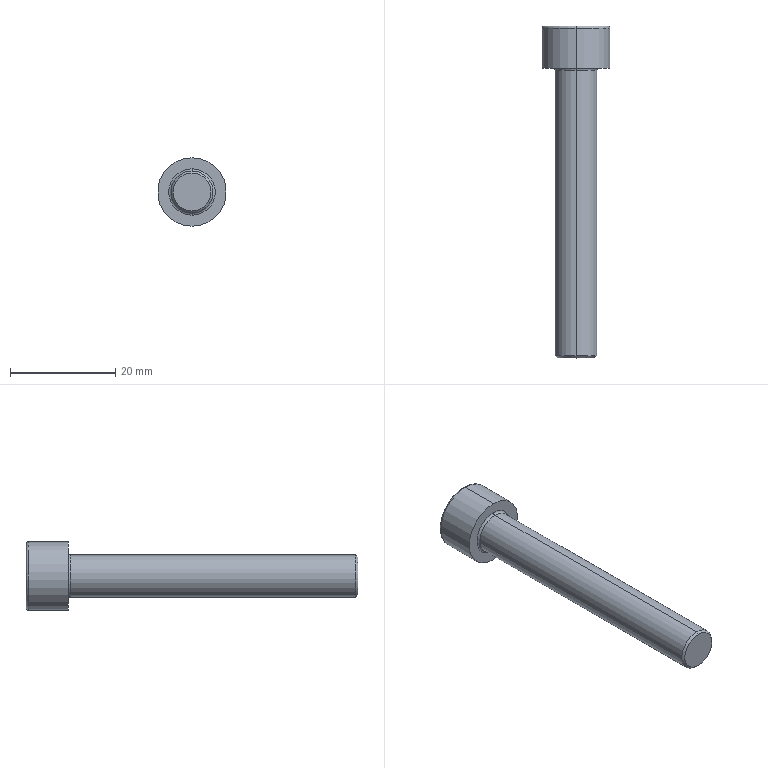Part | STEP file | 1 solid | 20 faces | box 13 x 63 x 13 mm | volume 3699 mm3 | plane 10 | torus 4 | cylinder 4 | cone 2 | commonest cylinder face diameters 8 x2 13 x2
STEP:
#1=CARTESIAN_POINT('',(0.,-55.,-3.6));
#2=VERTEX_POINT('',#1);
#3=CARTESIAN_POINT('',(0.,-55.,3.6));
#4=VERTEX_POINT('',#3);
#5=CARTESIAN_POINT('',(0.,-55.,0.));
#6=DIRECTION('',(0.,-1.,0.));
#7=DIRECTION('',(0.,0.,-1.));
#8=AXIS2_PLACEMENT_3D('',#5,#6,#7);
#9=CIRCLE('',#8,3.6);
#10=EDGE_CURVE('',#2,#4,#9,.T.);
#11=ORIENTED_EDGE('',*,*,#10,.F.);
#12=CARTESIAN_POINT('',(0.,-54.6,-4.));
#13=VERTEX_POINT('',#12);
#14=CARTESIAN_POINT('',(0.,-55.,-3.6));
#15=DIRECTION('',(0.,0.7071,-0.7071));
#16=VECTOR('',#15,1000.);
#17=LINE('',#14,#16);
#18=EDGE_CURVE('',#2,#13,#17,.T.);
#19=ORIENTED_EDGE('',*,*,#18,.T.);
#20=CARTESIAN_POINT('',(0.,-54.6,4.));
#21=VERTEX_POINT('',#20);
#22=CARTESIAN_POINT('',(0.,-54.6,0.));
#23=DIRECTION('',(0.,1.,0.));
#24=DIRECTION('',(0.,0.,-1.));
#25=AXIS2_PLACEMENT_3D('',#22,#23,#24);
#26=CIRCLE('',#25,4.);
#27=EDGE_CURVE('',#21,#13,#26,.T.);
#28=ORIENTED_EDGE('',*,*,#27,.F.);
#29=CARTESIAN_POINT('',(0.,-55.,3.6));
#30=DIRECTION('',(0.,0.7071,0.7071));
#31=VECTOR('',#30,1000.);
#32=LINE('',#29,#31);
#33=EDGE_CURVE('',#4,#21,#32,.T.);
#34=ORIENTED_EDGE('',*,*,#33,.F.);
#35=EDGE_LOOP('',(#11,#19,#28,#34));
#36=FACE_OUTER_BOUND('',#35,.T.);
#37=CARTESIAN_POINT('',(0.,-55.,0.));
#38=DIRECTION('',(0.,1.,0.));
#39=DIRECTION('',(0.,0.,1.));
#40=AXIS2_PLACEMENT_3D('',#37,#38,#39);
#41=CONICAL_SURFACE('',#40,3.6,0.7854);
#42=ADVANCED_FACE('',(#36),#41,.T.);
#43=CARTESIAN_POINT('',(0.,7.6,-6.5));
#44=VERTEX_POINT('',#43);
#45=CARTESIAN_POINT('',(0.,7.6,6.5));
#46=VERTEX_POINT('',#45);
#47=CARTESIAN_POINT('',(0.,7.6,0.));
#48=DIRECTION('',(0.,-1.,0.));
#49=DIRECTION('',(0.,0.,1.));
#50=AXIS2_PLACEMENT_3D('',#47,#48,#49);
#51=CIRCLE('',#50,6.5);
#52=EDGE_CURVE('',#44,#46,#51,.T.);
#53=ORIENTED_EDGE('',*,*,#52,.F.);
#54=CARTESIAN_POINT('',(0.,8.,-6.1));
#55=VERTEX_POINT('',#54);
#56=CARTESIAN_POINT('',(0.,7.6,-6.1));
#57=DIRECTION('',(1.,0.,0.));
#58=DIRECTION('',(0.,0.,-1.));
#59=AXIS2_PLACEMENT_3D('',#56,#57,#58);
#60=CIRCLE('',#59,0.4);
#61=EDGE_CURVE('',#44,#55,#60,.T.);
#62=ORIENTED_EDGE('',*,*,#61,.T.);
#63=CARTESIAN_POINT('',(0.,8.,6.1));
#64=VERTEX_POINT('',#63);
#65=CARTESIAN_POINT('',(0.,8.,0.));
#66=DIRECTION('',(0.,1.,0.));
#67=DIRECTION('',(0.,0.,1.));
#68=AXIS2_PLACEMENT_3D('',#65,#66,#67);
#69=CIRCLE('',#68,6.1);
#70=EDGE_CURVE('',#64,#55,#69,.T.);
#71=ORIENTED_EDGE('',*,*,#70,.F.);
#72=CARTESIAN_POINT('',(0.,7.6,6.1));
#73=DIRECTION('',(-1.,0.,0.));
#74=DIRECTION('',(0.,0.,1.));
#75=AXIS2_PLACEMENT_3D('',#72,#73,#74);
#76=CIRCLE('',#75,0.4);
#77=EDGE_CURVE('',#46,#64,#76,.T.);
#78=ORIENTED_EDGE('',*,*,#77,.F.);
#79=EDGE_LOOP('',(#53,#62,#71,#78));
#80=FACE_OUTER_BOUND('',#79,.T.);
#81=CARTESIAN_POINT('',(0.,7.6,0.));
#82=DIRECTION('',(0.,1.,0.));
#83=DIRECTION('',(0.,0.,1.));
#84=AXIS2_PLACEMENT_3D('',#81,#82,#83);
#85=TOROIDAL_SURFACE('',#84,6.1,0.4);
#86=ADVANCED_FACE('',(#80),#85,.T.);
#87=CARTESIAN_POINT('',(0.,-0.4,4.));
#88=VERTEX_POINT('',#87);
#89=CARTESIAN_POINT('',(0.,-0.4,-4.));
#90=VERTEX_POINT('',#89);
#91=CARTESIAN_POINT('',(0.,-0.4,0.));
#92=DIRECTION('',(0.,-1.,0.));
#93=DIRECTION('',(0.,0.,-1.));
#94=AXIS2_PLACEMENT_3D('',#91,#92,#93);
#95=CIRCLE('',#94,4.);
#96=EDGE_CURVE('',#88,#90,#95,.T.);
#97=ORIENTED_EDGE('',*,*,#96,.F.);
#98=CARTESIAN_POINT('',(0.,0.,4.4));
#99=VERTEX_POINT('',#98);
#100=CARTESIAN_POINT('',(0.,-0.4,4.4));
#101=DIRECTION('',(1.,0.,0.));
#102=DIRECTION('',(0.,0.,-1.));
#103=AXIS2_PLACEMENT_3D('',#100,#101,#102);
#104=CIRCLE('',#103,0.4);
#105=EDGE_CURVE('',#88,#99,#104,.T.);
#106=ORIENTED_EDGE('',*,*,#105,.T.);
#107=CARTESIAN_POINT('',(0.,0.,-4.4));
#108=VERTEX_POINT('',#107);
#109=CARTESIAN_POINT('',(0.,0.,0.));
#110=DIRECTION('',(0.,1.,0.));
#111=DIRECTION('',(0.,0.,-1.));
#112=AXIS2_PLACEMENT_3D('',#109,#110,#111);
#113=CIRCLE('',#112,4.4);
#114=EDGE_CURVE('',#108,#99,#113,.T.);
#115=ORIENTED_EDGE('',*,*,#114,.F.);
#116=CARTESIAN_POINT('',(0.,-0.4,-4.4));
#117=DIRECTION('',(-1.,0.,0.));
#118=DIRECTION('',(0.,0.,1.));
#119=AXIS2_PLACEMENT_3D('',#116,#117,#118);
#120=CIRCLE('',#119,0.4);
#121=EDGE_CURVE('',#90,#108,#120,.T.);
#122=ORIENTED_EDGE('',*,*,#121,.F.);
#123=EDGE_LOOP('',(#97,#106,#115,#122));
#124=FACE_OUTER_BOUND('',#123,.T.);
#125=CARTESIAN_POINT('',(0.,-0.4,0.));
#126=DIRECTION('',(0.,-1.,0.));
#127=DIRECTION('',(0.,0.,-1.));
#128=AXIS2_PLACEMENT_3D('',#125,#126,#127);
#129=TOROIDAL_SURFACE('',#128,4.4,0.4);
#130=ADVANCED_FACE('',(#124),#129,.F.);
#131=CARTESIAN_POINT('',(0.,-0.4,0.));
#132=DIRECTION('',(0.,-1.,0.));
#133=DIRECTION('',(0.,0.,-1.));
#134=AXIS2_PLACEMENT_3D('',#131,#132,#133);
#135=CIRCLE('',#134,4.);
#136=EDGE_CURVE('',#90,#88,#135,.T.);
#137=ORIENTED_EDGE('',*,*,#136,.T.);
#138=CARTESIAN_POINT('',(0.,0.,4.));
#139=DIRECTION('',(0.,-1.,0.));
#140=VECTOR('',#139,1000.);
#141=LINE('',#138,#140);
#142=EDGE_CURVE('',#88,#21,#141,.T.);
#143=ORIENTED_EDGE('',*,*,#142,.T.);
#144=ORIENTED_EDGE('',*,*,#27,.T.);
#145=CARTESIAN_POINT('',(0.,0.,-4.));
#146=DIRECTION('',(0.,-1.,0.));
#147=VECTOR('',#146,1000.);
#148=LINE('',#145,#147);
#149=EDGE_CURVE('',#90,#13,#148,.T.);
#150=ORIENTED_EDGE('',*,*,#149,.F.);
#151=EDGE_LOOP('',(#137,#143,#144,#150));
#152=FACE_OUTER_BOUND('',#151,.T.);
#153=CARTESIAN_POINT('',(0.,0.,0.));
#154=DIRECTION('',(0.,-1.,0.));
#155=DIRECTION('',(0.,0.,-1.));
#156=AXIS2_PLACEMENT_3D('',#153,#154,#155);
#157=CYLINDRICAL_SURFACE('',#156,4.);
#158=ADVANCED_FACE('',(#152),#157,.T.);
#159=ORIENTED_EDGE('',*,*,#52,.T.);
#160=CARTESIAN_POINT('',(0.,0.,6.5));
#161=VERTEX_POINT('',#160);
#162=CARTESIAN_POINT('',(0.,0.,6.5));
#163=DIRECTION('',(0.,-1.,0.));
#164=VECTOR('',#163,1000.);
#165=LINE('',#162,#164);
#166=EDGE_CURVE('',#46,#161,#165,.T.);
#167=ORIENTED_EDGE('',*,*,#166,.T.);
#168=CARTESIAN_POINT('',(0.,0.,-6.5));
#169=VERTEX_POINT('',#168);
#170=CARTESIAN_POINT('',(0.,0.,0.));
#171=DIRECTION('',(0.,-1.,0.));
#172=DIRECTION('',(0.,0.,-1.));
#173=AXIS2_PLACEMENT_3D('',#170,#171,#172);
#174=CIRCLE('',#173,6.5);
#175=EDGE_CURVE('',#169,#161,#174,.T.);
#176=ORIENTED_EDGE('',*,*,#175,.F.);
#177=CARTESIAN_POINT('',(0.,0.,-6.5));
#178=DIRECTION('',(0.,-1.,0.));
#179=VECTOR('',#178,1000.);
#180=LINE('',#177,#179);
#181=EDGE_CURVE('',#44,#169,#180,.T.);
#182=ORIENTED_EDGE('',*,*,#181,.F.);
#183=EDGE_LOOP('',(#159,#167,#176,#182));
#184=FACE_OUTER_BOUND('',#183,.T.);
#185=CARTESIAN_POINT('',(0.,0.,0.));
#186=DIRECTION('',(0.,-1.,0.));
#187=DIRECTION('',(0.,0.,-1.));
#188=AXIS2_PLACEMENT_3D('',#185,#186,#187);
#189=CYLINDRICAL_SURFACE('',#188,6.5);
#190=ADVANCED_FACE('',(#184),#189,.T.);
#191=ORIENTED_EDGE('',*,*,#70,.T.);
#192=CARTESIAN_POINT('',(0.,8.,0.));
#193=DIRECTION('',(0.,1.,0.));
#194=DIRECTION('',(0.,0.,1.));
#195=AXIS2_PLACEMENT_3D('',#192,#193,#194);
#196=CIRCLE('',#195,6.1);
#197=EDGE_CURVE('',#55,#64,#196,.T.);
#198=ORIENTED_EDGE('',*,*,#197,.T.);
#199=EDGE_LOOP('',(#191,#198));
#200=FACE_OUTER_BOUND('',#199,.T.);
#201=CARTESIAN_POINT('',(0.,8.,-3.464));
#202=VERTEX_POINT('',#201);
#203=CARTESIAN_POINT('',(-3.,8.,-1.732));
#204=VERTEX_POINT('',#203);
#205=CARTESIAN_POINT('',(0.,8.,-3.464));
#206=DIRECTION('',(-0.866,0.,0.5));
#207=VECTOR('',#206,1000.);
#208=LINE('',#205,#207);
#209=EDGE_CURVE('',#202,#204,#208,.T.);
#210=ORIENTED_EDGE('',*,*,#209,.F.);
#211=CARTESIAN_POINT('',(3.,8.,-1.732));
#212=VERTEX_POINT('',#211);
#213=CARTESIAN_POINT('',(3.,8.,-1.732));
#214=DIRECTION('',(-0.866,0.,-0.5));
#215=VECTOR('',#214,1000.);
#216=LINE('',#213,#215);
#217=EDGE_CURVE('',#212,#202,#216,.T.);
#218=ORIENTED_EDGE('',*,*,#217,.F.);
#219=CARTESIAN_POINT('',(3.,8.,1.732));
#220=VERTEX_POINT('',#219);
#221=CARTESIAN_POINT('',(3.,8.,1.732));
#222=DIRECTION('',(0.,0.,-1.));
#223=VECTOR('',#222,1000.);
#224=LINE('',#221,#223);
#225=EDGE_CURVE('',#220,#212,#224,.T.);
#226=ORIENTED_EDGE('',*,*,#225,.F.);
#227=CARTESIAN_POINT('',(0.,8.,3.464));
#228=VERTEX_POINT('',#227);
#229=CARTESIAN_POINT('',(0.,8.,3.464));
#230=DIRECTION('',(0.866,0.,-0.5));
#231=VECTOR('',#230,1000.);
#232=LINE('',#229,#231);
#233=EDGE_CURVE('',#228,#220,#232,.T.);
#234=ORIENTED_EDGE('',*,*,#233,.F.);
#235=CARTESIAN_POINT('',(-3.,8.,1.732));
#236=VERTEX_POINT('',#235);
#237=CARTESIAN_POINT('',(-3.,8.,1.732));
#238=DIRECTION('',(0.866,0.,0.5));
#239=VECTOR('',#238,1000.);
#240=LINE('',#237,#239);
#241=EDGE_CURVE('',#236,#228,#240,.T.);
#242=ORIENTED_EDGE('',*,*,#241,.F.);
#243=CARTESIAN_POINT('',(-3.,8.,-1.732));
#244=DIRECTION('',(0.,0.,1.));
#245=VECTOR('',#244,1000.);
#246=LINE('',#243,#245);
#247=EDGE_CURVE('',#204,#236,#246,.T.);
#248=ORIENTED_EDGE('',*,*,#247,.F.);
#249=EDGE_LOOP('',(#210,#218,#226,#234,#242,#248));
#250=FACE_BOUND('',#249,.T.);
#251=CARTESIAN_POINT('',(0.,8.,0.));
#252=DIRECTION('',(0.,1.,0.));
#253=DIRECTION('',(0.,0.,1.));
#254=AXIS2_PLACEMENT_3D('',#251,#252,#253);
#255=PLANE('',#254);
#256=ADVANCED_FACE('',(#200,#250),#255,.T.);
#257=ORIENTED_EDGE('',*,*,#166,.F.);
#258=CARTESIAN_POINT('',(0.,7.6,0.));
#259=DIRECTION('',(0.,-1.,0.));
#260=DIRECTION('',(0.,0.,1.));
#261=AXIS2_PLACEMENT_3D('',#258,#259,#260);
#262=CIRCLE('',#261,6.5);
#263=EDGE_CURVE('',#46,#44,#262,.T.);
#264=ORIENTED_EDGE('',*,*,#263,.T.);
#265=ORIENTED_EDGE('',*,*,#181,.T.);
#266=CARTESIAN_POINT('',(0.,0.,0.));
#267=DIRECTION('',(0.,-1.,0.));
#268=DIRECTION('',(0.,0.,-1.));
#269=AXIS2_PLACEMENT_3D('',#266,#267,#268);
#270=CIRCLE('',#269,6.5);
#271=EDGE_CURVE('',#161,#169,#270,.T.);
#272=ORIENTED_EDGE('',*,*,#271,.F.);
#273=EDGE_LOOP('',(#257,#264,#265,#272));
#274=FACE_OUTER_BOUND('',#273,.T.);
#275=CARTESIAN_POINT('',(0.,0.,0.));
#276=DIRECTION('',(0.,-1.,0.));
#277=DIRECTION('',(0.,0.,-1.));
#278=AXIS2_PLACEMENT_3D('',#275,#276,#277);
#279=CYLINDRICAL_SURFACE('',#278,6.5);
#280=ADVANCED_FACE('',(#274),#279,.T.);
#281=ORIENTED_EDGE('',*,*,#114,.T.);
#282=CARTESIAN_POINT('',(0.,0.,0.));
#283=DIRECTION('',(0.,1.,0.));
#284=DIRECTION('',(0.,0.,-1.));
#285=AXIS2_PLACEMENT_3D('',#282,#283,#284);
#286=CIRCLE('',#285,4.4);
#287=EDGE_CURVE('',#99,#108,#286,.T.);
#288=ORIENTED_EDGE('',*,*,#287,.T.);
#289=EDGE_LOOP('',(#281,#288));
#290=FACE_BOUND('',#289,.T.);
#291=ORIENTED_EDGE('',*,*,#175,.T.);
#292=ORIENTED_EDGE('',*,*,#271,.T.);
#293=EDGE_LOOP('',(#291,#292));
#294=FACE_OUTER_BOUND('',#293,.T.);
#295=CARTESIAN_POINT('',(6.5,0.,0.));
#296=DIRECTION('',(0.,-1.,0.));
#297=DIRECTION('',(0.,0.,-1.));
#298=AXIS2_PLACEMENT_3D('',#295,#296,#297);
#299=PLANE('',#298);
#300=ADVANCED_FACE('',(#290,#294),#299,.T.);
#301=ORIENTED_EDGE('',*,*,#142,.F.);
#302=ORIENTED_EDGE('',*,*,#96,.T.);
#303=ORIENTED_EDGE('',*,*,#149,.T.);
#304=CARTESIAN_POINT('',(0.,-54.6,0.));
#305=DIRECTION('',(0.,1.,0.));
#306=DIRECTION('',(0.,0.,-1.));
#307=AXIS2_PLACEMENT_3D('',#304,#305,#306);
#308=CIRCLE('',#307,4.);
#309=EDGE_CURVE('',#13,#21,#308,.T.);
#310=ORIENTED_EDGE('',*,*,#309,.T.);
#311=EDGE_LOOP('',(#301,#302,#303,#310));
#312=FACE_OUTER_BOUND('',#311,.T.);
#313=CARTESIAN_POINT('',(0.,0.,0.));
#314=DIRECTION('',(0.,-1.,0.));
#315=DIRECTION('',(0.,0.,-1.));
#316=AXIS2_PLACEMENT_3D('',#313,#314,#315);
#317=CYLINDRICAL_SURFACE('',#316,4.);
#318=ADVANCED_FACE('',(#312),#317,.T.);
#319=CARTESIAN_POINT('',(0.,-55.,0.));
#320=DIRECTION('',(0.,-1.,0.));
#321=DIRECTION('',(0.,0.,-1.));
#322=AXIS2_PLACEMENT_3D('',#319,#320,#321);
#323=CIRCLE('',#322,3.6);
#324=EDGE_CURVE('',#4,#2,#323,.T.);
#325=ORIENTED_EDGE('',*,*,#324,.T.);
#326=ORIENTED_EDGE('',*,*,#10,.T.);
#327=EDGE_LOOP('',(#325,#326));
#328=FACE_OUTER_BOUND('',#327,.T.);
#329=CARTESIAN_POINT('',(4.,-55.,0.));
#330=DIRECTION('',(0.,-1.,0.));
#331=DIRECTION('',(0.,0.,-1.));
#332=AXIS2_PLACEMENT_3D('',#329,#330,#331);
#333=PLANE('',#332);
#334=ADVANCED_FACE('',(#328),#333,.T.);
#335=ORIENTED_EDGE('',*,*,#209,.T.);
#336=CARTESIAN_POINT('',(-3.,4.,-1.732));
#337=VERTEX_POINT('',#336);
#338=CARTESIAN_POINT('',(-3.,4.,-1.732));
#339=DIRECTION('',(0.,1.,0.));
#340=VECTOR('',#339,1000.);
#341=LINE('',#338,#340);
#342=EDGE_CURVE('',#337,#204,#341,.T.);
#343=ORIENTED_EDGE('',*,*,#342,.F.);
#344=CARTESIAN_POINT('',(0.,4.,-3.464));
#345=VERTEX_POINT('',#344);
#346=CARTESIAN_POINT('',(0.,4.,-3.464));
#347=DIRECTION('',(-0.866,0.,0.5));
#348=VECTOR('',#347,1000.);
#349=LINE('',#346,#348);
#350=EDGE_CURVE('',#345,#337,#349,.T.);
#351=ORIENTED_EDGE('',*,*,#350,.F.);
#352=CARTESIAN_POINT('',(0.,4.,-3.464));
#353=DIRECTION('',(0.,1.,0.));
#354=VECTOR('',#353,1000.);
#355=LINE('',#352,#354);
#356=EDGE_CURVE('',#345,#202,#355,.T.);
#357=ORIENTED_EDGE('',*,*,#356,.T.);
#358=EDGE_LOOP('',(#335,#343,#351,#357));
#359=FACE_OUTER_BOUND('',#358,.T.);
#360=CARTESIAN_POINT('',(0.,4.,-3.464));
#361=DIRECTION('',(-0.5,0.,-0.866));
#362=DIRECTION('',(-0.866,0.,0.5));
#363=AXIS2_PLACEMENT_3D('',#360,#361,#362);
#364=PLANE('',#363);
#365=ADVANCED_FACE('',(#359),#364,.F.);
#366=ORIENTED_EDGE('',*,*,#217,.T.);
#367=ORIENTED_EDGE('',*,*,#356,.F.);
#368=CARTESIAN_POINT('',(3.,4.,-1.732));
#369=VERTEX_POINT('',#368);
#370=CARTESIAN_POINT('',(3.,4.,-1.732));
#371=DIRECTION('',(-0.866,0.,-0.5));
#372=VECTOR('',#371,1000.);
#373=LINE('',#370,#372);
#374=EDGE_CURVE('',#369,#345,#373,.T.);
#375=ORIENTED_EDGE('',*,*,#374,.F.);
#376=CARTESIAN_POINT('',(3.,4.,-1.732));
#377=DIRECTION('',(0.,1.,0.));
#378=VECTOR('',#377,1000.);
#379=LINE('',#376,#378);
#380=EDGE_CURVE('',#369,#212,#379,.T.);
#381=ORIENTED_EDGE('',*,*,#380,.T.);
#382=EDGE_LOOP('',(#366,#367,#375,#381));
#383=FACE_OUTER_BOUND('',#382,.T.);
#384=CARTESIAN_POINT('',(3.,4.,-1.732));
#385=DIRECTION('',(0.5,0.,-0.866));
#386=DIRECTION('',(-0.866,0.,-0.5));
#387=AXIS2_PLACEMENT_3D('',#384,#385,#386);
#388=PLANE('',#387);
#389=ADVANCED_FACE('',(#383),#388,.F.);
#390=ORIENTED_EDGE('',*,*,#225,.T.);
#391=ORIENTED_EDGE('',*,*,#380,.F.);
#392=CARTESIAN_POINT('',(3.,4.,1.732));
#393=VERTEX_POINT('',#392);
#394=CARTESIAN_POINT('',(3.,4.,1.732));
#395=DIRECTION('',(0.,0.,-1.));
#396=VECTOR('',#395,1000.);
#397=LINE('',#394,#396);
#398=EDGE_CURVE('',#393,#369,#397,.T.);
#399=ORIENTED_EDGE('',*,*,#398,.F.);
#400=CARTESIAN_POINT('',(3.,4.,1.732));
#401=DIRECTION('',(0.,1.,0.));
#402=VECTOR('',#401,1000.);
#403=LINE('',#400,#402);
#404=EDGE_CURVE('',#393,#220,#403,.T.);
#405=ORIENTED_EDGE('',*,*,#404,.T.);
#406=EDGE_LOOP('',(#390,#391,#399,#405));
#407=FACE_OUTER_BOUND('',#406,.T.);
#408=CARTESIAN_POINT('',(3.,4.,1.732));
#409=DIRECTION('',(1.,0.,0.));
#410=DIRECTION('',(0.,0.,-1.));
#411=AXIS2_PLACEMENT_3D('',#408,#409,#410);
#412=PLANE('',#411);
#413=ADVANCED_FACE('',(#407),#412,.F.);
#414=ORIENTED_EDGE('',*,*,#233,.T.);
#415=ORIENTED_EDGE('',*,*,#404,.F.);
#416=CARTESIAN_POINT('',(0.,4.,3.464));
#417=VERTEX_POINT('',#416);
#418=CARTESIAN_POINT('',(0.,4.,3.464));
#419=DIRECTION('',(0.866,0.,-0.5));
#420=VECTOR('',#419,1000.);
#421=LINE('',#418,#420);
#422=EDGE_CURVE('',#417,#393,#421,.T.);
#423=ORIENTED_EDGE('',*,*,#422,.F.);
#424=CARTESIAN_POINT('',(0.,4.,3.464));
#425=DIRECTION('',(0.,1.,0.));
#426=VECTOR('',#425,1000.);
#427=LINE('',#424,#426);
#428=EDGE_CURVE('',#417,#228,#427,.T.);
#429=ORIENTED_EDGE('',*,*,#428,.T.);
#430=EDGE_LOOP('',(#414,#415,#423,#429));
#431=FACE_OUTER_BOUND('',#430,.T.);
#432=CARTESIAN_POINT('',(0.,4.,3.464));
#433=DIRECTION('',(0.5,0.,0.866));
#434=DIRECTION('',(0.866,0.,-0.5));
#435=AXIS2_PLACEMENT_3D('',#432,#433,#434);
#436=PLANE('',#435);
#437=ADVANCED_FACE('',(#431),#436,.F.);
#438=ORIENTED_EDGE('',*,*,#241,.T.);
#439=ORIENTED_EDGE('',*,*,#428,.F.);
#440=CARTESIAN_POINT('',(-3.,4.,1.732));
#441=VERTEX_POINT('',#440);
#442=CARTESIAN_POINT('',(-3.,4.,1.732));
#443=DIRECTION('',(0.866,0.,0.5));
#444=VECTOR('',#443,1000.);
#445=LINE('',#442,#444);
#446=EDGE_CURVE('',#441,#417,#445,.T.);
#447=ORIENTED_EDGE('',*,*,#446,.F.);
#448=CARTESIAN_POINT('',(-3.,4.,1.732));
#449=DIRECTION('',(0.,1.,0.));
#450=VECTOR('',#449,1000.);
#451=LINE('',#448,#450);
#452=EDGE_CURVE('',#441,#236,#451,.T.);
#453=ORIENTED_EDGE('',*,*,#452,.T.);
#454=EDGE_LOOP('',(#438,#439,#447,#453));
#455=FACE_OUTER_BOUND('',#454,.T.);
#456=CARTESIAN_POINT('',(-3.,4.,1.732));
#457=DIRECTION('',(-0.5,0.,0.866));
#458=DIRECTION('',(0.866,0.,0.5));
#459=AXIS2_PLACEMENT_3D('',#456,#457,#458);
#460=PLANE('',#459);
#461=ADVANCED_FACE('',(#455),#460,.F.);
#462=ORIENTED_EDGE('',*,*,#247,.T.);
#463=ORIENTED_EDGE('',*,*,#452,.F.);
#464=CARTESIAN_POINT('',(-3.,4.,-1.732));
#465=DIRECTION('',(0.,0.,1.));
#466=VECTOR('',#465,1000.);
#467=LINE('',#464,#466);
#468=EDGE_CURVE('',#337,#441,#467,.T.);
#469=ORIENTED_EDGE('',*,*,#468,.F.);
#470=ORIENTED_EDGE('',*,*,#342,.T.);
#471=EDGE_LOOP('',(#462,#463,#469,#470));
#472=FACE_OUTER_BOUND('',#471,.T.);
#473=CARTESIAN_POINT('',(-3.,4.,-1.732));
#474=DIRECTION('',(-1.,0.,0.));
#475=DIRECTION('',(0.,0.,1.));
#476=AXIS2_PLACEMENT_3D('',#473,#474,#475);
#477=PLANE('',#476);
#478=ADVANCED_FACE('',(#472),#477,.F.);
#479=ORIENTED_EDGE('',*,*,#350,.T.);
#480=ORIENTED_EDGE('',*,*,#468,.T.);
#481=ORIENTED_EDGE('',*,*,#446,.T.);
#482=ORIENTED_EDGE('',*,*,#422,.T.);
#483=ORIENTED_EDGE('',*,*,#398,.T.);
#484=ORIENTED_EDGE('',*,*,#374,.T.);
#485=EDGE_LOOP('',(#479,#480,#481,#482,#483,#484));
#486=FACE_OUTER_BOUND('',#485,.T.);
#487=CARTESIAN_POINT('',(0.,4.,0.));
#488=DIRECTION('',(0.,1.,0.));
#489=DIRECTION('',(0.,0.,1.));
#490=AXIS2_PLACEMENT_3D('',#487,#488,#489);
#491=PLANE('',#490);
#492=ADVANCED_FACE('',(#486),#491,.T.);
#493=ORIENTED_EDGE('',*,*,#105,.F.);
#494=ORIENTED_EDGE('',*,*,#136,.F.);
#495=ORIENTED_EDGE('',*,*,#121,.T.);
#496=ORIENTED_EDGE('',*,*,#287,.F.);
#497=EDGE_LOOP('',(#493,#494,#495,#496));
#498=FACE_OUTER_BOUND('',#497,.T.);
#499=CARTESIAN_POINT('',(0.,-0.4,0.));
#500=DIRECTION('',(0.,-1.,0.));
#501=DIRECTION('',(0.,0.,-1.));
#502=AXIS2_PLACEMENT_3D('',#499,#500,#501);
#503=TOROIDAL_SURFACE('',#502,4.4,0.4);
#504=ADVANCED_FACE('',(#498),#503,.F.);
#505=ORIENTED_EDGE('',*,*,#61,.F.);
#506=ORIENTED_EDGE('',*,*,#263,.F.);
#507=ORIENTED_EDGE('',*,*,#77,.T.);
#508=ORIENTED_EDGE('',*,*,#197,.F.);
#509=EDGE_LOOP('',(#505,#506,#507,#508));
#510=FACE_OUTER_BOUND('',#509,.T.);
#511=CARTESIAN_POINT('',(0.,7.6,0.));
#512=DIRECTION('',(0.,1.,0.));
#513=DIRECTION('',(0.,0.,1.));
#514=AXIS2_PLACEMENT_3D('',#511,#512,#513);
#515=TOROIDAL_SURFACE('',#514,6.1,0.4);
#516=ADVANCED_FACE('',(#510),#515,.T.);
#517=ORIENTED_EDGE('',*,*,#18,.F.);
#518=ORIENTED_EDGE('',*,*,#324,.F.);
#519=ORIENTED_EDGE('',*,*,#33,.T.);
#520=ORIENTED_EDGE('',*,*,#309,.F.);
#521=EDGE_LOOP('',(#517,#518,#519,#520));
#522=FACE_OUTER_BOUND('',#521,.T.);
#523=CARTESIAN_POINT('',(0.,-55.,0.));
#524=DIRECTION('',(0.,1.,0.));
#525=DIRECTION('',(0.,0.,1.));
#526=AXIS2_PLACEMENT_3D('',#523,#524,#525);
#527=CONICAL_SURFACE('',#526,3.6,0.7854);
#528=ADVANCED_FACE('',(#522),#527,.T.);
#529=CLOSED_SHELL('',(#42,#86,#130,#158,#190,#256,#280,#300,#318,#334,#365,#389,#413,#437,#461,#478,#492,#504,#516,#528));
#530=MANIFOLD_SOLID_BREP('',#529);
#531=CARTESIAN_POINT('',(0.,0.,0.));
#532=DIRECTION('',(0.,0.,1.));
#533=DIRECTION('',(1.,0.,0.));
#534=AXIS2_PLACEMENT_3D('',#531,#532,#533);
#535=(LENGTH_UNIT()NAMED_UNIT(*)SI_UNIT(.MILLI.,.METRE.));
#536=UNCERTAINTY_MEASURE_WITH_UNIT(LENGTH_MEASURE(0.00001),#535,'','');
#537=(NAMED_UNIT(*)PLANE_ANGLE_UNIT()SI_UNIT($,.RADIAN.));
#538=(NAMED_UNIT(*)SI_UNIT($,.STERADIAN.)SOLID_ANGLE_UNIT());
#539=(GEOMETRIC_REPRESENTATION_CONTEXT(3)GLOBAL_UNCERTAINTY_ASSIGNED_CONTEXT((#536))GLOBAL_UNIT_ASSIGNED_CONTEXT((#535,#537,#538))REPRESENTATION_CONTEXT('',''));
#540=ADVANCED_BREP_SHAPE_REPRESENTATION('',(#530,#534),#539);